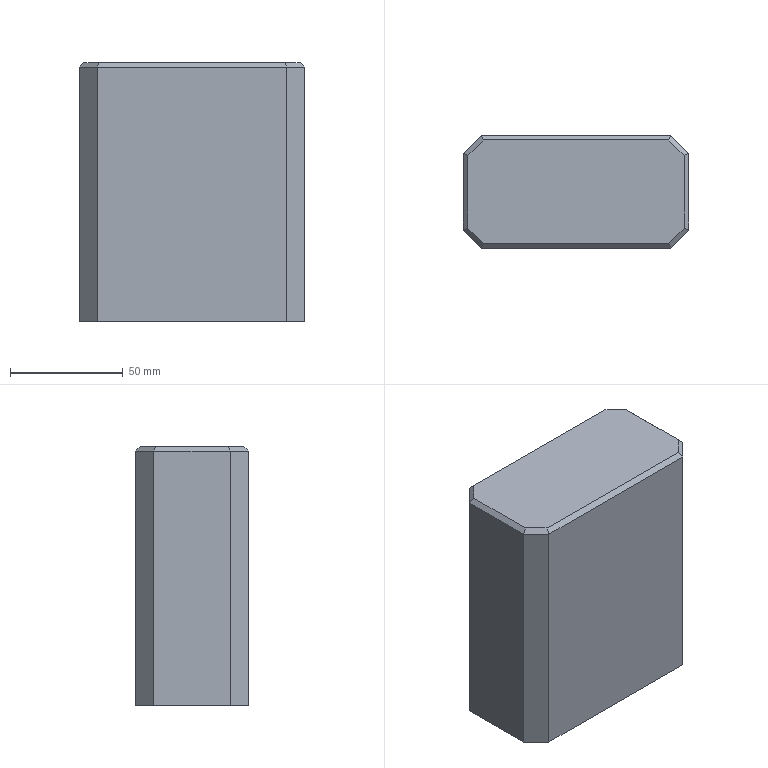Part | STEP file | TJ-DHQM-003-007 | 1 solid | 26 faces | box 100 x 50 x 115 mm | volume 555425 mm3 | plane 18 | cylinder 4 | cone 4 | commonest cylinder face diameters 10.2 x4
STEP:
#1=CARTESIAN_POINT('',(41.1,0.,25.3));
#2=VERTEX_POINT('',#1);
#3=CARTESIAN_POINT('',(30.9,0.,25.3));
#4=VERTEX_POINT('',#3);
#5=CARTESIAN_POINT('',(36.,0.,25.3));
#6=DIRECTION('',(0.,0.,-1.));
#7=DIRECTION('',(-1.,0.,0.));
#8=AXIS2_PLACEMENT_3D('',#5,#6,#7);
#9=CIRCLE('',#8,5.1);
#10=EDGE_CURVE('',#2,#4,#9,.T.);
#11=ORIENTED_EDGE('',*,*,#10,.F.);
#12=CARTESIAN_POINT('',(41.1,0.,0.));
#13=VERTEX_POINT('',#12);
#14=CARTESIAN_POINT('',(41.1,0.,0.));
#15=DIRECTION('',(0.,0.,-1.));
#16=VECTOR('',#15,1000.);
#17=LINE('',#14,#16);
#18=EDGE_CURVE('',#2,#13,#17,.T.);
#19=ORIENTED_EDGE('',*,*,#18,.T.);
#20=CARTESIAN_POINT('',(30.9,0.,0.));
#21=VERTEX_POINT('',#20);
#22=CARTESIAN_POINT('',(36.,0.,0.));
#23=DIRECTION('',(0.,0.,-1.));
#24=DIRECTION('',(-1.,0.,0.));
#25=AXIS2_PLACEMENT_3D('',#22,#23,#24);
#26=CIRCLE('',#25,5.1);
#27=EDGE_CURVE('',#13,#21,#26,.T.);
#28=ORIENTED_EDGE('',*,*,#27,.T.);
#29=CARTESIAN_POINT('',(30.9,0.,0.));
#30=DIRECTION('',(0.,0.,-1.));
#31=VECTOR('',#30,1000.);
#32=LINE('',#29,#31);
#33=EDGE_CURVE('',#4,#21,#32,.T.);
#34=ORIENTED_EDGE('',*,*,#33,.F.);
#35=EDGE_LOOP('',(#11,#19,#28,#34));
#36=FACE_OUTER_BOUND('',#35,.T.);
#37=CARTESIAN_POINT('',(36.,0.,0.));
#38=DIRECTION('',(0.,0.,-1.));
#39=DIRECTION('',(-1.,0.,0.));
#40=AXIS2_PLACEMENT_3D('',#37,#38,#39);
#41=CYLINDRICAL_SURFACE('',#40,5.1);
#42=ADVANCED_FACE('',(#36),#41,.F.);
#43=CARTESIAN_POINT('',(36.,0.,28.364));
#44=VERTEX_POINT('',#43);
#45=CARTESIAN_POINT('',(30.9,0.,25.3));
#46=DIRECTION('',(-0.8572,0.,-0.515));
#47=VECTOR('',#46,1000.);
#48=LINE('',#45,#47);
#49=EDGE_CURVE('',#44,#4,#48,.T.);
#50=ORIENTED_EDGE('',*,*,#49,.F.);
#51=CARTESIAN_POINT('',(41.1,0.,25.3));
#52=DIRECTION('',(0.8572,0.,-0.515));
#53=VECTOR('',#52,1000.);
#54=LINE('',#51,#53);
#55=EDGE_CURVE('',#44,#2,#54,.T.);
#56=ORIENTED_EDGE('',*,*,#55,.T.);
#57=ORIENTED_EDGE('',*,*,#10,.T.);
#58=EDGE_LOOP('',(#50,#56,#57));
#59=FACE_OUTER_BOUND('',#58,.T.);
#60=CARTESIAN_POINT('',(36.,0.,25.3));
#61=DIRECTION('',(0.,0.,-1.));
#62=DIRECTION('',(-1.,0.,0.));
#63=AXIS2_PLACEMENT_3D('',#60,#61,#62);
#64=CONICAL_SURFACE('',#63,5.1,1.03);
#65=ADVANCED_FACE('',(#59),#64,.F.);
#66=CARTESIAN_POINT('',(-30.9,0.,25.3));
#67=VERTEX_POINT('',#66);
#68=CARTESIAN_POINT('',(-41.1,0.,25.3));
#69=VERTEX_POINT('',#68);
#70=CARTESIAN_POINT('',(-36.,0.,25.3));
#71=DIRECTION('',(0.,0.,-1.));
#72=DIRECTION('',(-1.,0.,0.));
#73=AXIS2_PLACEMENT_3D('',#70,#71,#72);
#74=CIRCLE('',#73,5.1);
#75=EDGE_CURVE('',#67,#69,#74,.T.);
#76=ORIENTED_EDGE('',*,*,#75,.F.);
#77=CARTESIAN_POINT('',(-30.9,0.,0.));
#78=VERTEX_POINT('',#77);
#79=CARTESIAN_POINT('',(-30.9,0.,0.));
#80=DIRECTION('',(0.,0.,-1.));
#81=VECTOR('',#80,1000.);
#82=LINE('',#79,#81);
#83=EDGE_CURVE('',#67,#78,#82,.T.);
#84=ORIENTED_EDGE('',*,*,#83,.T.);
#85=CARTESIAN_POINT('',(-41.1,0.,0.));
#86=VERTEX_POINT('',#85);
#87=CARTESIAN_POINT('',(-36.,0.,0.));
#88=DIRECTION('',(0.,0.,-1.));
#89=DIRECTION('',(-1.,0.,0.));
#90=AXIS2_PLACEMENT_3D('',#87,#88,#89);
#91=CIRCLE('',#90,5.1);
#92=EDGE_CURVE('',#78,#86,#91,.T.);
#93=ORIENTED_EDGE('',*,*,#92,.T.);
#94=CARTESIAN_POINT('',(-41.1,0.,0.));
#95=DIRECTION('',(0.,0.,-1.));
#96=VECTOR('',#95,1000.);
#97=LINE('',#94,#96);
#98=EDGE_CURVE('',#69,#86,#97,.T.);
#99=ORIENTED_EDGE('',*,*,#98,.F.);
#100=EDGE_LOOP('',(#76,#84,#93,#99));
#101=FACE_OUTER_BOUND('',#100,.T.);
#102=CARTESIAN_POINT('',(-36.,0.,0.));
#103=DIRECTION('',(0.,0.,-1.));
#104=DIRECTION('',(-1.,0.,0.));
#105=AXIS2_PLACEMENT_3D('',#102,#103,#104);
#106=CYLINDRICAL_SURFACE('',#105,5.1);
#107=ADVANCED_FACE('',(#101),#106,.F.);
#108=CARTESIAN_POINT('',(-36.,0.,28.364));
#109=VERTEX_POINT('',#108);
#110=CARTESIAN_POINT('',(-41.1,0.,25.3));
#111=DIRECTION('',(-0.8572,0.,-0.515));
#112=VECTOR('',#111,1000.);
#113=LINE('',#110,#112);
#114=EDGE_CURVE('',#109,#69,#113,.T.);
#115=ORIENTED_EDGE('',*,*,#114,.F.);
#116=CARTESIAN_POINT('',(-30.9,0.,25.3));
#117=DIRECTION('',(0.8572,0.,-0.515));
#118=VECTOR('',#117,1000.);
#119=LINE('',#116,#118);
#120=EDGE_CURVE('',#109,#67,#119,.T.);
#121=ORIENTED_EDGE('',*,*,#120,.T.);
#122=ORIENTED_EDGE('',*,*,#75,.T.);
#123=EDGE_LOOP('',(#115,#121,#122));
#124=FACE_OUTER_BOUND('',#123,.T.);
#125=CARTESIAN_POINT('',(-36.,0.,25.3));
#126=DIRECTION('',(0.,0.,-1.));
#127=DIRECTION('',(-1.,0.,0.));
#128=AXIS2_PLACEMENT_3D('',#125,#126,#127);
#129=CONICAL_SURFACE('',#128,5.1,1.03);
#130=ADVANCED_FACE('',(#124),#129,.F.);
#131=CARTESIAN_POINT('',(50.,17.,0.));
#132=VERTEX_POINT('',#131);
#133=CARTESIAN_POINT('',(50.,17.,113.));
#134=VERTEX_POINT('',#133);
#135=CARTESIAN_POINT('',(50.,17.,115.));
#136=DIRECTION('',(0.,0.,1.));
#137=VECTOR('',#136,1000.);
#138=LINE('',#135,#137);
#139=EDGE_CURVE('',#132,#134,#138,.T.);
#140=ORIENTED_EDGE('',*,*,#139,.T.);
#141=CARTESIAN_POINT('',(50.,-17.,113.));
#142=VERTEX_POINT('',#141);
#143=CARTESIAN_POINT('',(50.,-17.,113.));
#144=DIRECTION('',(0.,-1.,0.));
#145=VECTOR('',#144,1000.);
#146=LINE('',#143,#145);
#147=EDGE_CURVE('',#134,#142,#146,.T.);
#148=ORIENTED_EDGE('',*,*,#147,.T.);
#149=CARTESIAN_POINT('',(50.,-17.,0.));
#150=VERTEX_POINT('',#149);
#151=CARTESIAN_POINT('',(50.,-17.,115.));
#152=DIRECTION('',(0.,0.,-1.));
#153=VECTOR('',#152,1000.);
#154=LINE('',#151,#153);
#155=EDGE_CURVE('',#142,#150,#154,.T.);
#156=ORIENTED_EDGE('',*,*,#155,.T.);
#157=CARTESIAN_POINT('',(50.,25.,0.));
#158=DIRECTION('',(0.,1.,0.));
#159=VECTOR('',#158,1000.);
#160=LINE('',#157,#159);
#161=EDGE_CURVE('',#150,#132,#160,.T.);
#162=ORIENTED_EDGE('',*,*,#161,.T.);
#163=EDGE_LOOP('',(#140,#148,#156,#162));
#164=FACE_OUTER_BOUND('',#163,.T.);
#165=CARTESIAN_POINT('',(50.,25.,115.));
#166=DIRECTION('',(-1.,0.,0.));
#167=DIRECTION('',(0.,-1.,0.));
#168=AXIS2_PLACEMENT_3D('',#165,#166,#167);
#169=PLANE('',#168);
#170=ADVANCED_FACE('',(#164),#169,.F.);
#171=CARTESIAN_POINT('',(-42.,25.,0.));
#172=VERTEX_POINT('',#171);
#173=CARTESIAN_POINT('',(-42.,25.,113.));
#174=VERTEX_POINT('',#173);
#175=CARTESIAN_POINT('',(-42.,25.,115.));
#176=DIRECTION('',(0.,0.,1.));
#177=VECTOR('',#176,1000.);
#178=LINE('',#175,#177);
#179=EDGE_CURVE('',#172,#174,#178,.T.);
#180=ORIENTED_EDGE('',*,*,#179,.T.);
#181=CARTESIAN_POINT('',(42.,25.,113.));
#182=VERTEX_POINT('',#181);
#183=CARTESIAN_POINT('',(42.,25.,113.));
#184=DIRECTION('',(1.,0.,0.));
#185=VECTOR('',#184,1000.);
#186=LINE('',#183,#185);
#187=EDGE_CURVE('',#174,#182,#186,.T.);
#188=ORIENTED_EDGE('',*,*,#187,.T.);
#189=CARTESIAN_POINT('',(42.,25.,0.));
#190=VERTEX_POINT('',#189);
#191=CARTESIAN_POINT('',(42.,25.,115.));
#192=DIRECTION('',(0.,0.,-1.));
#193=VECTOR('',#192,1000.);
#194=LINE('',#191,#193);
#195=EDGE_CURVE('',#182,#190,#194,.T.);
#196=ORIENTED_EDGE('',*,*,#195,.T.);
#197=CARTESIAN_POINT('',(-50.,25.,0.));
#198=DIRECTION('',(-1.,0.,0.));
#199=VECTOR('',#198,1000.);
#200=LINE('',#197,#199);
#201=EDGE_CURVE('',#190,#172,#200,.T.);
#202=ORIENTED_EDGE('',*,*,#201,.T.);
#203=EDGE_LOOP('',(#180,#188,#196,#202));
#204=FACE_OUTER_BOUND('',#203,.T.);
#205=CARTESIAN_POINT('',(-50.,25.,115.));
#206=DIRECTION('',(0.,-1.,0.));
#207=DIRECTION('',(0.,0.,-1.));
#208=AXIS2_PLACEMENT_3D('',#205,#206,#207);
#209=PLANE('',#208);
#210=ADVANCED_FACE('',(#204),#209,.F.);
#211=CARTESIAN_POINT('',(-50.,-17.,0.));
#212=VERTEX_POINT('',#211);
#213=CARTESIAN_POINT('',(-50.,-17.,113.));
#214=VERTEX_POINT('',#213);
#215=CARTESIAN_POINT('',(-50.,-17.,115.));
#216=DIRECTION('',(0.,0.,1.));
#217=VECTOR('',#216,1000.);
#218=LINE('',#215,#217);
#219=EDGE_CURVE('',#212,#214,#218,.T.);
#220=ORIENTED_EDGE('',*,*,#219,.T.);
#221=CARTESIAN_POINT('',(-50.,17.,113.));
#222=VERTEX_POINT('',#221);
#223=CARTESIAN_POINT('',(-50.,17.,113.));
#224=DIRECTION('',(0.,1.,0.));
#225=VECTOR('',#224,1000.);
#226=LINE('',#223,#225);
#227=EDGE_CURVE('',#214,#222,#226,.T.);
#228=ORIENTED_EDGE('',*,*,#227,.T.);
#229=CARTESIAN_POINT('',(-50.,17.,0.));
#230=VERTEX_POINT('',#229);
#231=CARTESIAN_POINT('',(-50.,17.,115.));
#232=DIRECTION('',(0.,0.,-1.));
#233=VECTOR('',#232,1000.);
#234=LINE('',#231,#233);
#235=EDGE_CURVE('',#222,#230,#234,.T.);
#236=ORIENTED_EDGE('',*,*,#235,.T.);
#237=CARTESIAN_POINT('',(-50.,25.,0.));
#238=DIRECTION('',(0.,-1.,0.));
#239=VECTOR('',#238,1000.);
#240=LINE('',#237,#239);
#241=EDGE_CURVE('',#230,#212,#240,.T.);
#242=ORIENTED_EDGE('',*,*,#241,.T.);
#243=EDGE_LOOP('',(#220,#228,#236,#242));
#244=FACE_OUTER_BOUND('',#243,.T.);
#245=CARTESIAN_POINT('',(-50.,25.,115.));
#246=DIRECTION('',(1.,0.,0.));
#247=DIRECTION('',(0.,1.,0.));
#248=AXIS2_PLACEMENT_3D('',#245,#246,#247);
#249=PLANE('',#248);
#250=ADVANCED_FACE('',(#244),#249,.F.);
#251=CARTESIAN_POINT('',(42.,-25.,0.));
#252=VERTEX_POINT('',#251);
#253=CARTESIAN_POINT('',(42.,-25.,113.));
#254=VERTEX_POINT('',#253);
#255=CARTESIAN_POINT('',(42.,-25.,115.));
#256=DIRECTION('',(0.,0.,1.));
#257=VECTOR('',#256,1000.);
#258=LINE('',#255,#257);
#259=EDGE_CURVE('',#252,#254,#258,.T.);
#260=ORIENTED_EDGE('',*,*,#259,.T.);
#261=CARTESIAN_POINT('',(-42.,-25.,113.));
#262=VERTEX_POINT('',#261);
#263=CARTESIAN_POINT('',(-42.,-25.,113.));
#264=DIRECTION('',(-1.,0.,0.));
#265=VECTOR('',#264,1000.);
#266=LINE('',#263,#265);
#267=EDGE_CURVE('',#254,#262,#266,.T.);
#268=ORIENTED_EDGE('',*,*,#267,.T.);
#269=CARTESIAN_POINT('',(-42.,-25.,0.));
#270=VERTEX_POINT('',#269);
#271=CARTESIAN_POINT('',(-42.,-25.,115.));
#272=DIRECTION('',(0.,0.,-1.));
#273=VECTOR('',#272,1000.);
#274=LINE('',#271,#273);
#275=EDGE_CURVE('',#262,#270,#274,.T.);
#276=ORIENTED_EDGE('',*,*,#275,.T.);
#277=CARTESIAN_POINT('',(-50.,-25.,0.));
#278=DIRECTION('',(1.,0.,0.));
#279=VECTOR('',#278,1000.);
#280=LINE('',#277,#279);
#281=EDGE_CURVE('',#270,#252,#280,.T.);
#282=ORIENTED_EDGE('',*,*,#281,.T.);
#283=EDGE_LOOP('',(#260,#268,#276,#282));
#284=FACE_OUTER_BOUND('',#283,.T.);
#285=CARTESIAN_POINT('',(-50.,-25.,115.));
#286=DIRECTION('',(0.,1.,0.));
#287=DIRECTION('',(0.,0.,1.));
#288=AXIS2_PLACEMENT_3D('',#285,#286,#287);
#289=PLANE('',#288);
#290=ADVANCED_FACE('',(#284),#289,.F.);
#291=CARTESIAN_POINT('',(48.,-16.172,115.));
#292=VERTEX_POINT('',#291);
#293=CARTESIAN_POINT('',(48.,16.172,115.));
#294=VERTEX_POINT('',#293);
#295=CARTESIAN_POINT('',(48.,17.,115.));
#296=DIRECTION('',(0.,1.,0.));
#297=VECTOR('',#296,1000.);
#298=LINE('',#295,#297);
#299=EDGE_CURVE('',#292,#294,#298,.T.);
#300=ORIENTED_EDGE('',*,*,#299,.T.);
#301=CARTESIAN_POINT('',(41.172,23.,115.));
#302=VERTEX_POINT('',#301);
#303=CARTESIAN_POINT('',(32.086,32.086,115.));
#304=DIRECTION('',(-0.7071,0.7071,0.));
#305=VECTOR('',#304,1000.);
#306=LINE('',#303,#305);
#307=EDGE_CURVE('',#294,#302,#306,.T.);
#308=ORIENTED_EDGE('',*,*,#307,.T.);
#309=CARTESIAN_POINT('',(-41.172,23.,115.));
#310=VERTEX_POINT('',#309);
#311=CARTESIAN_POINT('',(-42.,23.,115.));
#312=DIRECTION('',(-1.,0.,0.));
#313=VECTOR('',#312,1000.);
#314=LINE('',#311,#313);
#315=EDGE_CURVE('',#302,#310,#314,.T.);
#316=ORIENTED_EDGE('',*,*,#315,.T.);
#317=CARTESIAN_POINT('',(-48.,16.172,115.));
#318=VERTEX_POINT('',#317);
#319=CARTESIAN_POINT('',(-32.086,32.086,115.));
#320=DIRECTION('',(-0.7071,-0.7071,0.));
#321=VECTOR('',#320,1000.);
#322=LINE('',#319,#321);
#323=EDGE_CURVE('',#310,#318,#322,.T.);
#324=ORIENTED_EDGE('',*,*,#323,.T.);
#325=CARTESIAN_POINT('',(-48.,-16.172,115.));
#326=VERTEX_POINT('',#325);
#327=CARTESIAN_POINT('',(-48.,-17.,115.));
#328=DIRECTION('',(0.,-1.,0.));
#329=VECTOR('',#328,1000.);
#330=LINE('',#327,#329);
#331=EDGE_CURVE('',#318,#326,#330,.T.);
#332=ORIENTED_EDGE('',*,*,#331,.T.);
#333=CARTESIAN_POINT('',(-41.172,-23.,115.));
#334=VERTEX_POINT('',#333);
#335=CARTESIAN_POINT('',(-32.086,-32.086,115.));
#336=DIRECTION('',(0.7071,-0.7071,0.));
#337=VECTOR('',#336,1000.);
#338=LINE('',#335,#337);
#339=EDGE_CURVE('',#326,#334,#338,.T.);
#340=ORIENTED_EDGE('',*,*,#339,.T.);
#341=CARTESIAN_POINT('',(41.172,-23.,115.));
#342=VERTEX_POINT('',#341);
#343=CARTESIAN_POINT('',(42.,-23.,115.));
#344=DIRECTION('',(1.,0.,0.));
#345=VECTOR('',#344,1000.);
#346=LINE('',#343,#345);
#347=EDGE_CURVE('',#334,#342,#346,.T.);
#348=ORIENTED_EDGE('',*,*,#347,.T.);
#349=CARTESIAN_POINT('',(32.086,-32.086,115.));
#350=DIRECTION('',(0.7071,0.7071,0.));
#351=VECTOR('',#350,1000.);
#352=LINE('',#349,#351);
#353=EDGE_CURVE('',#342,#292,#352,.T.);
#354=ORIENTED_EDGE('',*,*,#353,.T.);
#355=EDGE_LOOP('',(#300,#308,#316,#324,#332,#340,#348,#354));
#356=FACE_OUTER_BOUND('',#355,.T.);
#357=CARTESIAN_POINT('',(0.,0.,115.));
#358=DIRECTION('',(0.,0.,1.));
#359=DIRECTION('',(1.,0.,0.));
#360=AXIS2_PLACEMENT_3D('',#357,#358,#359);
#361=PLANE('',#360);
#362=ADVANCED_FACE('',(#356),#361,.T.);
#363=CARTESIAN_POINT('',(36.,0.,0.));
#364=DIRECTION('',(0.,0.,-1.));
#365=DIRECTION('',(-1.,0.,0.));
#366=AXIS2_PLACEMENT_3D('',#363,#364,#365);
#367=CIRCLE('',#366,5.1);
#368=EDGE_CURVE('',#21,#13,#367,.T.);
#369=ORIENTED_EDGE('',*,*,#368,.F.);
#370=ORIENTED_EDGE('',*,*,#27,.F.);
#371=EDGE_LOOP('',(#369,#370));
#372=FACE_BOUND('',#371,.T.);
#373=CARTESIAN_POINT('',(-36.,0.,0.));
#374=DIRECTION('',(0.,0.,-1.));
#375=DIRECTION('',(-1.,0.,0.));
#376=AXIS2_PLACEMENT_3D('',#373,#374,#375);
#377=CIRCLE('',#376,5.1);
#378=EDGE_CURVE('',#86,#78,#377,.T.);
#379=ORIENTED_EDGE('',*,*,#378,.F.);
#380=ORIENTED_EDGE('',*,*,#92,.F.);
#381=EDGE_LOOP('',(#379,#380));
#382=FACE_BOUND('',#381,.T.);
#383=ORIENTED_EDGE('',*,*,#241,.F.);
#384=CARTESIAN_POINT('',(-50.,17.,0.));
#385=DIRECTION('',(0.7071,0.7071,0.));
#386=VECTOR('',#385,1000.);
#387=LINE('',#384,#386);
#388=EDGE_CURVE('',#230,#172,#387,.T.);
#389=ORIENTED_EDGE('',*,*,#388,.T.);
#390=ORIENTED_EDGE('',*,*,#201,.F.);
#391=CARTESIAN_POINT('',(42.,25.,0.));
#392=DIRECTION('',(0.7071,-0.7071,0.));
#393=VECTOR('',#392,1000.);
#394=LINE('',#391,#393);
#395=EDGE_CURVE('',#190,#132,#394,.T.);
#396=ORIENTED_EDGE('',*,*,#395,.T.);
#397=ORIENTED_EDGE('',*,*,#161,.F.);
#398=CARTESIAN_POINT('',(50.,-17.,0.));
#399=DIRECTION('',(-0.7071,-0.7071,0.));
#400=VECTOR('',#399,1000.);
#401=LINE('',#398,#400);
#402=EDGE_CURVE('',#150,#252,#401,.T.);
#403=ORIENTED_EDGE('',*,*,#402,.T.);
#404=ORIENTED_EDGE('',*,*,#281,.F.);
#405=CARTESIAN_POINT('',(-42.,-25.,0.));
#406=DIRECTION('',(-0.7071,0.7071,0.));
#407=VECTOR('',#406,1000.);
#408=LINE('',#405,#407);
#409=EDGE_CURVE('',#270,#212,#408,.T.);
#410=ORIENTED_EDGE('',*,*,#409,.T.);
#411=EDGE_LOOP('',(#383,#389,#390,#396,#397,#403,#404,#410));
#412=FACE_OUTER_BOUND('',#411,.T.);
#413=CARTESIAN_POINT('',(0.,0.,0.));
#414=DIRECTION('',(0.,0.,1.));
#415=DIRECTION('',(1.,0.,0.));
#416=AXIS2_PLACEMENT_3D('',#413,#414,#415);
#417=PLANE('',#416);
#418=ADVANCED_FACE('',(#372,#382,#412),#417,.F.);
#419=ORIENTED_EDGE('',*,*,#235,.F.);
#420=CARTESIAN_POINT('',(-50.,17.,113.));
#421=DIRECTION('',(0.7071,0.7071,0.));
#422=VECTOR('',#421,1000.);
#423=LINE('',#420,#422);
#424=EDGE_CURVE('',#222,#174,#423,.T.);
#425=ORIENTED_EDGE('',*,*,#424,.T.);
#426=ORIENTED_EDGE('',*,*,#179,.F.);
#427=ORIENTED_EDGE('',*,*,#388,.F.);
#428=EDGE_LOOP('',(#419,#425,#426,#427));
#429=FACE_OUTER_BOUND('',#428,.T.);
#430=CARTESIAN_POINT('',(-50.,17.,115.));
#431=DIRECTION('',(0.7071,-0.7071,0.));
#432=DIRECTION('',(0.,0.,-1.));
#433=AXIS2_PLACEMENT_3D('',#430,#431,#432);
#434=PLANE('',#433);
#435=ADVANCED_FACE('',(#429),#434,.F.);
#436=ORIENTED_EDGE('',*,*,#195,.F.);
#437=CARTESIAN_POINT('',(42.,25.,113.));
#438=DIRECTION('',(0.7071,-0.7071,0.));
#439=VECTOR('',#438,1000.);
#440=LINE('',#437,#439);
#441=EDGE_CURVE('',#182,#134,#440,.T.);
#442=ORIENTED_EDGE('',*,*,#441,.T.);
#443=ORIENTED_EDGE('',*,*,#139,.F.);
#444=ORIENTED_EDGE('',*,*,#395,.F.);
#445=EDGE_LOOP('',(#436,#442,#443,#444));
#446=FACE_OUTER_BOUND('',#445,.T.);
#447=CARTESIAN_POINT('',(42.,25.,115.));
#448=DIRECTION('',(-0.7071,-0.7071,0.));
#449=DIRECTION('',(0.,0.,-1.));
#450=AXIS2_PLACEMENT_3D('',#447,#448,#449);
#451=PLANE('',#450);
#452=ADVANCED_FACE('',(#446),#451,.F.);
#453=ORIENTED_EDGE('',*,*,#155,.F.);
#454=CARTESIAN_POINT('',(50.,-17.,113.));
#455=DIRECTION('',(-0.7071,-0.7071,0.));
#456=VECTOR('',#455,1000.);
#457=LINE('',#454,#456);
#458=EDGE_CURVE('',#142,#254,#457,.T.);
#459=ORIENTED_EDGE('',*,*,#458,.T.);
#460=ORIENTED_EDGE('',*,*,#259,.F.);
#461=ORIENTED_EDGE('',*,*,#402,.F.);
#462=EDGE_LOOP('',(#453,#459,#460,#461));
#463=FACE_OUTER_BOUND('',#462,.T.);
#464=CARTESIAN_POINT('',(50.,-17.,115.));
#465=DIRECTION('',(-0.7071,0.7071,0.));
#466=DIRECTION('',(0.,0.,-1.));
#467=AXIS2_PLACEMENT_3D('',#464,#465,#466);
#468=PLANE('',#467);
#469=ADVANCED_FACE('',(#463),#468,.F.);
#470=ORIENTED_EDGE('',*,*,#275,.F.);
#471=CARTESIAN_POINT('',(-42.,-25.,113.));
#472=DIRECTION('',(-0.7071,0.7071,0.));
#473=VECTOR('',#472,1000.);
#474=LINE('',#471,#473);
#475=EDGE_CURVE('',#262,#214,#474,.T.);
#476=ORIENTED_EDGE('',*,*,#475,.T.);
#477=ORIENTED_EDGE('',*,*,#219,.F.);
#478=ORIENTED_EDGE('',*,*,#409,.F.);
#479=EDGE_LOOP('',(#470,#476,#477,#478));
#480=FACE_OUTER_BOUND('',#479,.T.);
#481=CARTESIAN_POINT('',(-42.,-25.,115.));
#482=DIRECTION('',(0.7071,0.7071,0.));
#483=DIRECTION('',(0.,0.,-1.));
#484=AXIS2_PLACEMENT_3D('',#481,#482,#483);
#485=PLANE('',#484);
#486=ADVANCED_FACE('',(#480),#485,.F.);
#487=CARTESIAN_POINT('',(-44.915,-14.894,118.085));
#488=DIRECTION('',(0.6786,0.2811,0.6786));
#489=VECTOR('',#488,1000.);
#490=LINE('',#487,#489);
#491=EDGE_CURVE('',#214,#326,#490,.T.);
#492=ORIENTED_EDGE('',*,*,#491,.F.);
#493=ORIENTED_EDGE('',*,*,#475,.F.);
#494=CARTESIAN_POINT('',(-42.187,-25.451,112.549));
#495=DIRECTION('',(-0.2811,-0.6786,-0.6786));
#496=VECTOR('',#495,1000.);
#497=LINE('',#494,#496);
#498=EDGE_CURVE('',#334,#262,#497,.T.);
#499=ORIENTED_EDGE('',*,*,#498,.F.);
#500=ORIENTED_EDGE('',*,*,#339,.F.);
#501=EDGE_LOOP('',(#492,#493,#499,#500));
#502=FACE_OUTER_BOUND('',#501,.T.);
#503=CARTESIAN_POINT('',(-32.086,-32.086,115.));
#504=DIRECTION('',(-0.5,-0.5,0.7071));
#505=DIRECTION('',(-0.7071,0.7071,0.));
#506=AXIS2_PLACEMENT_3D('',#503,#504,#505);
#507=PLANE('',#506);
#508=ADVANCED_FACE('',(#502),#507,.T.);
#509=ORIENTED_EDGE('',*,*,#498,.T.);
#510=ORIENTED_EDGE('',*,*,#267,.F.);
#511=CARTESIAN_POINT('',(37.919,-15.147,122.853));
#512=DIRECTION('',(0.2811,-0.6786,-0.6786));
#513=VECTOR('',#512,1000.);
#514=LINE('',#511,#513);
#515=EDGE_CURVE('',#342,#254,#514,.T.);
#516=ORIENTED_EDGE('',*,*,#515,.F.);
#517=ORIENTED_EDGE('',*,*,#347,.F.);
#518=EDGE_LOOP('',(#509,#510,#516,#517));
#519=FACE_OUTER_BOUND('',#518,.T.);
#520=CARTESIAN_POINT('',(0.,-23.,115.));
#521=DIRECTION('',(0.,-0.7071,0.7071));
#522=DIRECTION('',(-1.,0.,0.));
#523=AXIS2_PLACEMENT_3D('',#520,#521,#522);
#524=PLANE('',#523);
#525=ADVANCED_FACE('',(#519),#524,.T.);
#526=ORIENTED_EDGE('',*,*,#491,.T.);
#527=ORIENTED_EDGE('',*,*,#331,.F.);
#528=CARTESIAN_POINT('',(-43.707,14.393,119.293));
#529=DIRECTION('',(0.6786,-0.2811,0.6786));
#530=VECTOR('',#529,1000.);
#531=LINE('',#528,#530);
#532=EDGE_CURVE('',#222,#318,#531,.T.);
#533=ORIENTED_EDGE('',*,*,#532,.F.);
#534=ORIENTED_EDGE('',*,*,#227,.F.);
#535=EDGE_LOOP('',(#526,#527,#533,#534));
#536=FACE_OUTER_BOUND('',#535,.T.);
#537=CARTESIAN_POINT('',(-48.,0.,115.));
#538=DIRECTION('',(-0.7071,0.,0.7071));
#539=DIRECTION('',(0.,1.,0.));
#540=AXIS2_PLACEMENT_3D('',#537,#538,#539);
#541=PLANE('',#540);
#542=ADVANCED_FACE('',(#536),#541,.T.);
#543=ORIENTED_EDGE('',*,*,#515,.T.);
#544=ORIENTED_EDGE('',*,*,#458,.F.);
#545=CARTESIAN_POINT('',(43.707,-14.393,119.293));
#546=DIRECTION('',(0.6786,-0.2811,-0.6786));
#547=VECTOR('',#546,1000.);
#548=LINE('',#545,#547);
#549=EDGE_CURVE('',#292,#142,#548,.T.);
#550=ORIENTED_EDGE('',*,*,#549,.F.);
#551=ORIENTED_EDGE('',*,*,#353,.F.);
#552=EDGE_LOOP('',(#543,#544,#550,#551));
#553=FACE_OUTER_BOUND('',#552,.T.);
#554=CARTESIAN_POINT('',(32.086,-32.086,115.));
#555=DIRECTION('',(0.5,-0.5,0.7071));
#556=DIRECTION('',(-0.7071,-0.7071,0.));
#557=AXIS2_PLACEMENT_3D('',#554,#555,#556);
#558=PLANE('',#557);
#559=ADVANCED_FACE('',(#553),#558,.T.);
#560=ORIENTED_EDGE('',*,*,#532,.T.);
#561=ORIENTED_EDGE('',*,*,#323,.F.);
#562=CARTESIAN_POINT('',(-37.919,15.147,122.853));
#563=DIRECTION('',(0.2811,-0.6786,0.6786));
#564=VECTOR('',#563,1000.);
#565=LINE('',#562,#564);
#566=EDGE_CURVE('',#174,#310,#565,.T.);
#567=ORIENTED_EDGE('',*,*,#566,.F.);
#568=ORIENTED_EDGE('',*,*,#424,.F.);
#569=EDGE_LOOP('',(#560,#561,#567,#568));
#570=FACE_OUTER_BOUND('',#569,.T.);
#571=CARTESIAN_POINT('',(-32.086,32.086,115.));
#572=DIRECTION('',(-0.5,0.5,0.7071));
#573=DIRECTION('',(0.7071,0.7071,0.));
#574=AXIS2_PLACEMENT_3D('',#571,#572,#573);
#575=PLANE('',#574);
#576=ADVANCED_FACE('',(#570),#575,.T.);
#577=ORIENTED_EDGE('',*,*,#549,.T.);
#578=ORIENTED_EDGE('',*,*,#147,.F.);
#579=CARTESIAN_POINT('',(44.915,14.894,118.085));
#580=DIRECTION('',(0.6786,0.2811,-0.6786));
#581=VECTOR('',#580,1000.);
#582=LINE('',#579,#581);
#583=EDGE_CURVE('',#294,#134,#582,.T.);
#584=ORIENTED_EDGE('',*,*,#583,.F.);
#585=ORIENTED_EDGE('',*,*,#299,.F.);
#586=EDGE_LOOP('',(#577,#578,#584,#585));
#587=FACE_OUTER_BOUND('',#586,.T.);
#588=CARTESIAN_POINT('',(48.,0.,115.));
#589=DIRECTION('',(0.7071,0.,0.7071));
#590=DIRECTION('',(0.,-1.,0.));
#591=AXIS2_PLACEMENT_3D('',#588,#589,#590);
#592=PLANE('',#591);
#593=ADVANCED_FACE('',(#587),#592,.T.);
#594=ORIENTED_EDGE('',*,*,#566,.T.);
#595=ORIENTED_EDGE('',*,*,#315,.F.);
#596=CARTESIAN_POINT('',(37.919,15.147,122.853));
#597=DIRECTION('',(-0.2811,-0.6786,0.6786));
#598=VECTOR('',#597,1000.);
#599=LINE('',#596,#598);
#600=EDGE_CURVE('',#182,#302,#599,.T.);
#601=ORIENTED_EDGE('',*,*,#600,.F.);
#602=ORIENTED_EDGE('',*,*,#187,.F.);
#603=EDGE_LOOP('',(#594,#595,#601,#602));
#604=FACE_OUTER_BOUND('',#603,.T.);
#605=CARTESIAN_POINT('',(0.,23.,115.));
#606=DIRECTION('',(0.,0.7071,0.7071));
#607=DIRECTION('',(1.,0.,0.));
#608=AXIS2_PLACEMENT_3D('',#605,#606,#607);
#609=PLANE('',#608);
#610=ADVANCED_FACE('',(#604),#609,.T.);
#611=ORIENTED_EDGE('',*,*,#583,.T.);
#612=ORIENTED_EDGE('',*,*,#441,.F.);
#613=ORIENTED_EDGE('',*,*,#600,.T.);
#614=ORIENTED_EDGE('',*,*,#307,.F.);
#615=EDGE_LOOP('',(#611,#612,#613,#614));
#616=FACE_OUTER_BOUND('',#615,.T.);
#617=CARTESIAN_POINT('',(32.086,32.086,115.));
#618=DIRECTION('',(0.5,0.5,0.7071));
#619=DIRECTION('',(0.7071,-0.7071,0.));
#620=AXIS2_PLACEMENT_3D('',#617,#618,#619);
#621=PLANE('',#620);
#622=ADVANCED_FACE('',(#616),#621,.T.);
#623=ORIENTED_EDGE('',*,*,#120,.F.);
#624=ORIENTED_EDGE('',*,*,#114,.T.);
#625=CARTESIAN_POINT('',(-36.,0.,25.3));
#626=DIRECTION('',(0.,0.,-1.));
#627=DIRECTION('',(-1.,0.,0.));
#628=AXIS2_PLACEMENT_3D('',#625,#626,#627);
#629=CIRCLE('',#628,5.1);
#630=EDGE_CURVE('',#69,#67,#629,.T.);
#631=ORIENTED_EDGE('',*,*,#630,.T.);
#632=EDGE_LOOP('',(#623,#624,#631));
#633=FACE_OUTER_BOUND('',#632,.T.);
#634=CARTESIAN_POINT('',(-36.,0.,25.3));
#635=DIRECTION('',(0.,0.,-1.));
#636=DIRECTION('',(-1.,0.,0.));
#637=AXIS2_PLACEMENT_3D('',#634,#635,#636);
#638=CONICAL_SURFACE('',#637,5.1,1.03);
#639=ADVANCED_FACE('',(#633),#638,.F.);
#640=ORIENTED_EDGE('',*,*,#83,.F.);
#641=ORIENTED_EDGE('',*,*,#630,.F.);
#642=ORIENTED_EDGE('',*,*,#98,.T.);
#643=ORIENTED_EDGE('',*,*,#378,.T.);
#644=EDGE_LOOP('',(#640,#641,#642,#643));
#645=FACE_OUTER_BOUND('',#644,.T.);
#646=CARTESIAN_POINT('',(-36.,0.,0.));
#647=DIRECTION('',(0.,0.,-1.));
#648=DIRECTION('',(-1.,0.,0.));
#649=AXIS2_PLACEMENT_3D('',#646,#647,#648);
#650=CYLINDRICAL_SURFACE('',#649,5.1);
#651=ADVANCED_FACE('',(#645),#650,.F.);
#652=ORIENTED_EDGE('',*,*,#55,.F.);
#653=ORIENTED_EDGE('',*,*,#49,.T.);
#654=CARTESIAN_POINT('',(36.,0.,25.3));
#655=DIRECTION('',(0.,0.,-1.));
#656=DIRECTION('',(-1.,0.,0.));
#657=AXIS2_PLACEMENT_3D('',#654,#655,#656);
#658=CIRCLE('',#657,5.1);
#659=EDGE_CURVE('',#4,#2,#658,.T.);
#660=ORIENTED_EDGE('',*,*,#659,.T.);
#661=EDGE_LOOP('',(#652,#653,#660));
#662=FACE_OUTER_BOUND('',#661,.T.);
#663=CARTESIAN_POINT('',(36.,0.,25.3));
#664=DIRECTION('',(0.,0.,-1.));
#665=DIRECTION('',(-1.,0.,0.));
#666=AXIS2_PLACEMENT_3D('',#663,#664,#665);
#667=CONICAL_SURFACE('',#666,5.1,1.03);
#668=ADVANCED_FACE('',(#662),#667,.F.);
#669=ORIENTED_EDGE('',*,*,#18,.F.);
#670=ORIENTED_EDGE('',*,*,#659,.F.);
#671=ORIENTED_EDGE('',*,*,#33,.T.);
#672=ORIENTED_EDGE('',*,*,#368,.T.);
#673=EDGE_LOOP('',(#669,#670,#671,#672));
#674=FACE_OUTER_BOUND('',#673,.T.);
#675=CARTESIAN_POINT('',(36.,0.,0.));
#676=DIRECTION('',(0.,0.,-1.));
#677=DIRECTION('',(-1.,0.,0.));
#678=AXIS2_PLACEMENT_3D('',#675,#676,#677);
#679=CYLINDRICAL_SURFACE('',#678,5.1);
#680=ADVANCED_FACE('',(#674),#679,.F.);
#681=CLOSED_SHELL('',(#42,#65,#107,#130,#170,#210,#250,#290,#362,#418,#435,#452,#469,#486,#508,#525,#542,#559,#576,#593,#610,#622,#639,#651,#668,#680));
#682=MANIFOLD_SOLID_BREP('',#681);
#683=CARTESIAN_POINT('',(0.,0.,0.));
#684=DIRECTION('',(0.,0.,1.));
#685=DIRECTION('',(1.,0.,0.));
#686=AXIS2_PLACEMENT_3D('',#683,#684,#685);
#687=(LENGTH_UNIT()NAMED_UNIT(*)SI_UNIT(.MILLI.,.METRE.));
#688=UNCERTAINTY_MEASURE_WITH_UNIT(LENGTH_MEASURE(0.00001),#687,'','');
#689=(NAMED_UNIT(*)PLANE_ANGLE_UNIT()SI_UNIT($,.RADIAN.));
#690=(NAMED_UNIT(*)SI_UNIT($,.STERADIAN.)SOLID_ANGLE_UNIT());
#691=(GEOMETRIC_REPRESENTATION_CONTEXT(3)GLOBAL_UNCERTAINTY_ASSIGNED_CONTEXT((#688))GLOBAL_UNIT_ASSIGNED_CONTEXT((#687,#689,#690))REPRESENTATION_CONTEXT('',''));
#692=ADVANCED_BREP_SHAPE_REPRESENTATION('',(#682,#686),#691);